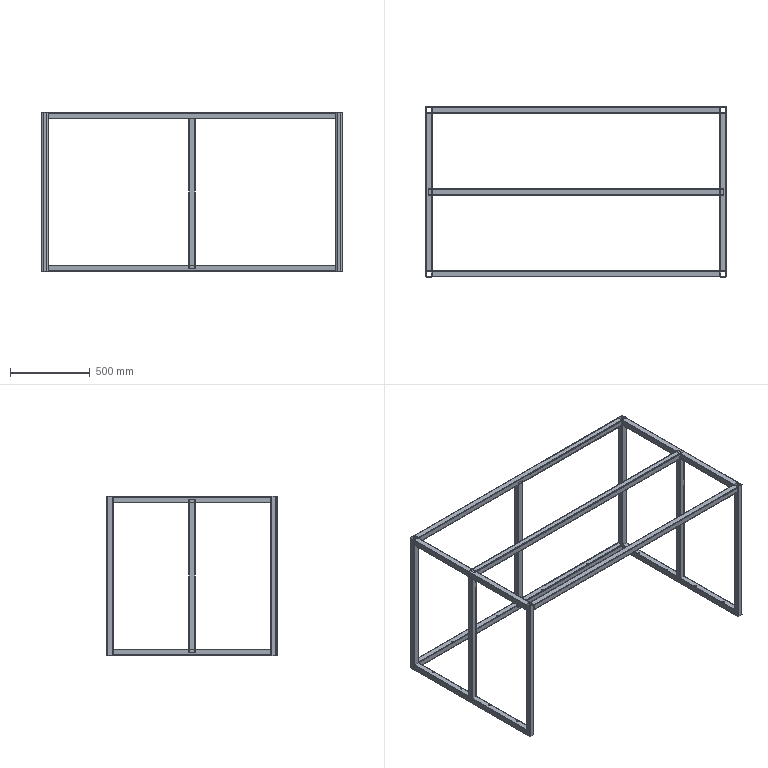Part | SolidWorks | features WeldCornerFeat 11, WeldMemberFeat 7, 3DProfileFeature 5, LPattern 3, HoleWzd 2, WeldmentFeature 1 | 15 solids | 318 faces | box 1890 x 1070 x 1000 mm | volume 5800253 mm3 | cylinder 168 | plane 150 | commonest cylinder face diameters 8 x60 4 x52 10 x48 16 x8